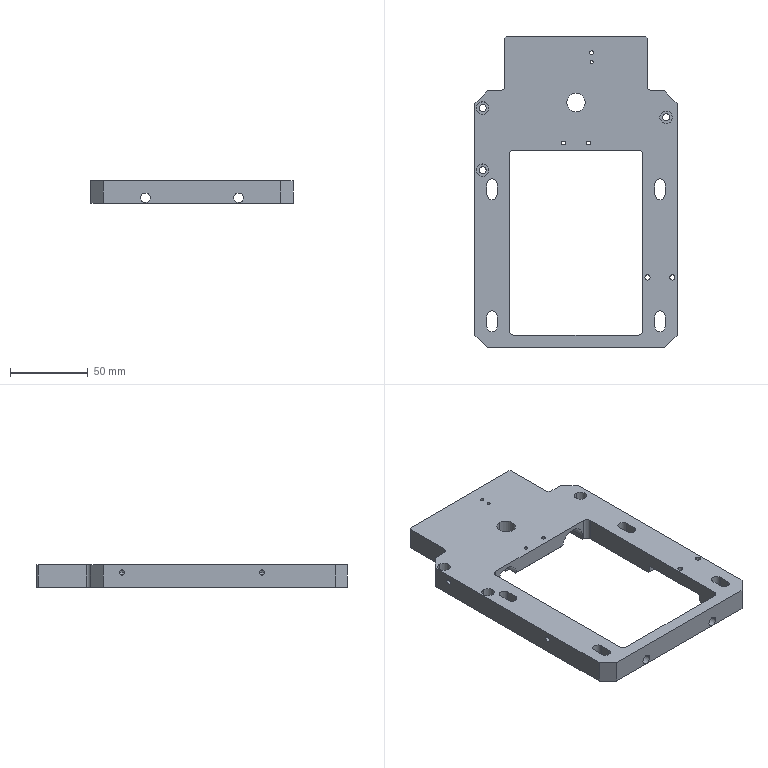NC program | NX | posted with a generic post | part box 130 x 200 x 14.5 mm
Lines 88 to 1425 of 25347:
(ZLEVEL_PROFILE_1_COPY , TOOL : D10)
N144 T04 M6
N146 G54
N148 G17 G0 G90 X12. Y-4.438 B0. C0. S3500 M3
N150 G43 Z30. H4
N152 Z1.5
N154 G94 G1 Y27.952 Z-0.197 F1000.
N156 X12.002 Y28. Z-0.2
N158 X-73.964 F2200.
N160 X-73.976 Y28.003
N162 X-74.442 Y28.002
N164 X-74.46 Y28.004
N166 X-74.993 Y28.
N168 X-77.
N170 Y-28.
N172 X12.002
N174 X12.003 Y-26.135
N176 X12. Y-26.122
N178 Y27.952
N180 X12.002 Y28.
N182 X0.544 Z-0.4
N184 X-73.964
N186 X-73.976 Y28.003
N188 X-74.442 Y28.002
N190 X-74.46 Y28.004
N192 X-74.993 Y28.
N194 X-77.
N196 Y-28.
N198 X12.002
N200 X12.003 Y-26.135
N202 X12. Y-26.122
N204 Y27.952
N206 X12.002 Y28.
N208 X0.544 Z-0.6
N210 X-73.964
N212 X-73.976 Y28.003
N214 X-74.442 Y28.002
N216 X-74.46 Y28.004
N218 X-74.993 Y28.
N220 X-77.
N222 Y-28.
N224 X12.002
N226 X12.003 Y-26.135
N228 X12. Y-26.122
N230 Y27.952
N232 X12.002 Y28.
N234 X0.544 Z-0.8
N236 X-73.964
N238 X-73.976 Y28.003
N240 X-74.442 Y28.002
N242 X-74.46 Y28.004
N244 X-74.993 Y28.
N246 X-77.
N248 Y-28.
N250 X12.002
N252 X12.003 Y-26.135
N254 X12. Y-26.122
N256 Y27.952
N258 X12.002 Y28.
N260 X0.544 Z-1.
N262 X-73.964
N264 X-73.976 Y28.003
N266 X-74.442 Y28.002
N268 X-74.46 Y28.004
N270 X-74.993 Y28.
N272 X-77.
N274 Y-28.
N276 X12.002
N278 X12.003 Y-26.135
N280 X12. Y-26.122
N282 Y27.952
N284 X12.002 Y28.
N286 X0.544 Z-1.2
N288 X-77.
N290 Y-28.
N292 X12.002
N294 X12.003 Y-26.135
N296 X12. Y-26.122
N298 Y27.952
N300 X12.002 Y28.
N302 X0.544 Z-1.4
N304 X-77.
N306 Y-28.
N308 X12.002
N310 X12.003 Y-26.135
N312 X12. Y-26.122
N314 Y27.952
N316 X12.002 Y28.
N318 X0.544 Z-1.6
N320 X-77.
N322 Y-28.
N324 X12.002
N326 X12.003 Y-26.135
N328 X12. Y-26.122
N330 Y27.952
N332 X12.002 Y28.
N334 X0.544 Z-1.8
N336 X-77.
N338 Y-28.
N340 X12.002
N342 X12.003 Y-26.135
N344 X12. Y-26.122
N346 Y27.952
N348 X12.002 Y28.
N350 X0.544 Z-2.
N352 X-77.
N354 Y-28.
N356 X12.002
N358 X12.003 Y-26.135
N360 X12. Y-26.122
N362 Y27.952
N364 X12.002 Y28.
N366 X0.544 Z-2.2
N368 X-77.
N370 Y-28.
N372 X12.002
N374 X12.003 Y-26.135
N376 X12. Y-26.122
N378 Y27.952
N380 X12.002 Y28.
N382 X0.544 Z-2.4
N384 X-77.
N386 Y-28.
N388 X12.002
N390 X12.003 Y-26.135
N392 X12. Y-26.122
N394 Y27.952
N396 X12.002 Y28.
N398 X0.544 Z-2.6
N400 X-77.
N402 Y-28.
N404 X12.002
N406 X12.003 Y-26.135
N408 X12. Y-26.122
N410 Y27.952
N412 X12.002 Y28.
N414 X0.544 Z-2.8
N416 X-77.
N418 Y-28.
N420 X12.002
N422 X12.003 Y-26.135
N424 X12. Y-26.122
N426 Y27.952
N428 X12.002 Y28.
N430 X0.544 Z-3.
N432 X-77.
N434 Y-28.
N436 X12.002
N438 X12.003 Y-26.135
N440 X12. Y-26.122
N442 Y27.952
N444 X12.002 Y28.
N446 X0.544 Z-3.2
N448 X-77.
N450 Y-28.
N452 X12.002
N454 X12.003 Y-26.135
N456 X12. Y-26.122
N458 Y27.952
N460 X12.002 Y28.
N462 X0.544 Z-3.4
N464 X-77.
N466 Y-28.
N468 X12.002
N470 X12.003 Y-26.135
N472 X12. Y-26.122
N474 Y27.952
N476 X12.002 Y28.
N478 X0.544 Z-3.6
N480 X-77.
N482 Y-28.
N484 X12.002
N486 X12.003 Y-26.135
N488 X12. Y-26.122
N490 Y27.952
N492 X12.002 Y28.
N494 X0.544 Z-3.8
N496 X-77.
N498 Y-28.
N500 X12.002
N502 X12.003 Y-26.135
N504 X12. Y-26.122
N506 Y27.952
N508 X12.002 Y28.
N510 X0.544 Z-4.
N512 X-77.
N514 Y-28.
N516 X12.002
N518 X12.003 Y-26.135
N520 X12. Y-26.122
N522 Y27.952
N524 X12.002 Y28.
N526 X0.544 Z-4.2
N528 X-77.
N530 Y-28.
N532 X12.002
N534 X12.003 Y-26.135
N536 X12. Y-26.122
N538 Y27.952
N540 X12.002 Y28.
N542 X0.544 Z-4.4
N544 X-77.
N546 Y-28.
N548 X12.002
N550 X12.003 Y-26.135
N552 X12. Y-26.122
N554 Y27.952
N556 X12.002 Y28.
N558 X0.544 Z-4.6
N560 X-77.
N562 Y-28.
N564 X12.002
N566 X12.003 Y-26.135
N568 X12. Y-26.122
N570 Y27.952
N572 X12.002 Y28.
N574 X0.544 Z-4.8
N576 X-77.
N578 Y-28.
N580 X12.002
N582 X12.003 Y-26.135
N584 X12. Y-26.122
N586 Y27.952
N588 X12.002 Y28.
N590 X0.544 Z-5.
N592 X-77.
N594 Y-28.
N596 X12.002
N598 X12.003 Y-26.135
N600 X12. Y-26.122
N602 Y27.952
N604 X12.002 Y28.
N606 X0.544 Z-5.2
N608 X-77.
N610 Y-28.
N612 X12.002
N614 X12.003 Y-26.135
N616 X12. Y-26.122
N618 Y27.952
N620 X12.002 Y28.
N622 X0.544 Z-5.4
N624 X-77.
N626 Y-28.
N628 X12.002
N630 X12.003 Y-26.135
N632 X12. Y-26.122
N634 Y27.952
N636 X12.002 Y28.
N638 X0.544 Z-5.6
N640 X-77.
N642 Y-28.
N644 X12.002
N646 X12.003 Y-26.135
N648 X12. Y-26.122
N650 Y27.952
N652 X12.002 Y28.
N654 X0.544 Z-5.8
N656 X-77.
N658 Y-28.
N660 X12.002
N662 X12.003 Y-26.135
N664 X12. Y-26.122
N666 Y27.952
N668 X12.002 Y28.
N670 X0.544 Z-6.
N672 X-77.
N674 Y-28.
N676 X12.002
N678 X12.003 Y-26.135
N680 X12. Y-26.122
N682 Y27.952
N684 X12.002 Y28.
N686 X0.544 Z-6.2
N688 X-77.
N690 Y-28.
N692 X12.002
N694 X12.003 Y-26.135
N696 X12. Y-26.122
N698 Y27.952
N700 X12.002 Y28.
N702 X0.544 Z-6.4
N704 X-77.
N706 Y-28.
N708 X12.002
N710 X12.003 Y-26.135
N712 X12. Y-26.122
N714 Y27.952
N716 X12.002 Y28.
N718 X0.544 Z-6.6
N720 X-77.
N722 Y-28.
N724 X12.002
N726 X12.003 Y-26.135
N728 X12. Y-26.122
N730 Y27.952
N732 X12.002 Y28.
N734 X0.544 Z-6.8
N736 X-77.
N738 Y-28.
N740 X12.002
N742 X12.003 Y-26.135
N744 X12. Y-26.122
N746 Y27.952
N748 X12.002 Y28.
N750 X0.544 Z-7.
N752 X-77.
N754 Y-28.
N756 X12.002
N758 X12.003 Y-26.135
N760 X12. Y-26.122
N762 Y27.952
N764 X12.002 Y28.
N766 X0.544 Z-7.2
N768 X-77.
N770 Y-28.
N772 X12.002
N774 X12.003 Y-26.135
N776 X12. Y-26.122
N778 Y27.952
N780 X12.002 Y28.
N782 X0.544 Z-7.4
N784 X-77.
N786 Y-28.
N788 X12.002
N790 X12.003 Y-26.135
N792 X12. Y-26.122
N794 Y27.952
N796 X12.002 Y28.
N798 X0.544 Z-7.6
N800 X-77.
N802 Y-28.
N804 X12.002
N806 X12.003 Y-26.135
N808 X12. Y-26.122
N810 Y27.952
N812 X12.002 Y28.
N814 X0.544 Z-7.8
N816 X-77.
N818 Y-28.
N820 X12.002
N822 X12.003 Y-26.135
N824 X12. Y-26.122
N826 Y27.952
N828 X12.002 Y28.
N830 X0.544 Z-8.
N832 X-77.
N834 Y-28.
N836 X12.002
N838 X12.003 Y-26.135
N840 X12. Y-26.122
N842 Y27.952
N844 X12.002 Y28.
N846 X0.544 Z-8.2
N848 X-77.
N850 Y-28.
N852 X12.002
N854 X12.003 Y-26.135
N856 X12. Y-26.122
N858 Y27.952
N860 X12.002 Y28.
N862 X0.544 Z-8.4
N864 X-77.
N866 Y-28.
N868 X12.002
N870 X12.003 Y-26.135
N872 X12. Y-26.122
N874 Y27.952
N876 X12.002 Y28.
N878 X0.544 Z-8.6
N880 X-77.
N882 Y-28.
N884 X12.002
N886 X12.003 Y-26.135
N888 X12. Y-26.122
N890 Y27.952
N892 X12.002 Y28.
N894 X0.544 Z-8.8
N896 X-77.
N898 Y-28.
N900 X12.002
N902 X12.003 Y-26.135
N904 X12. Y-26.122
N906 Y27.952
N908 X12.002 Y28.
N910 X0.544 Z-9.
N912 X-77.
N914 Y-28.
N916 X12.002
N918 X12.003 Y-26.135
N920 X12. Y-26.122
N922 Y27.952
N924 X12.002 Y28.
N926 X0.544 Z-9.2
N928 X-77.
N930 Y-28.
N932 X12.002
N934 X12.003 Y-26.135
N936 X12. Y-26.122
N938 Y27.952
N940 X12.002 Y28.
N942 X0.544 Z-9.4
N944 X-77.
N946 Y-28.
N948 X12.002
N950 X12.003 Y-26.135
N952 X12. Y-26.122
N954 Y27.952
N956 X12.002 Y28.
N958 X0.544 Z-9.6
N960 X-77.
N962 Y-28.
N964 X12.002
N966 Y-26.135
N968 X12. Y-26.122
N970 Y27.952
N972 X12.002 Y28.
N974 X0.544 Z-9.8
N976 X-77.
N978 Y-28.
N980 X12.002
N982 Y-26.135
N984 X12. Y-26.122
N986 Y27.952
N988 X12.002 Y28.
N990 X0.544 Z-10.
N992 X-77.
N994 Y-28.
N996 X12.002
N998 Y-26.135
N1000 X12. Y-26.122
N1002 Y27.952
N1004 X12.002 Y28.
N1006 X0.544 Z-10.2
N1008 X-77.
N1010 Y-28.
N1012 X12.002
N1014 Y-26.135
N1016 X12. Y-26.122
N1018 Y27.952
N1020 X12.002 Y28.
N1022 X0.544 Z-10.4
N1024 X-77.
N1026 Y-28.
N1028 X12.002
N1030 Y-26.135
N1032 X12. Y-26.122
N1034 Y27.952
N1036 X12.002 Y28.
N1038 X0.544 Z-10.6
N1040 X-77.
N1042 Y-28.
N1044 X12.002
N1046 Y-26.135
N1048 X12. Y-26.122
N1050 Y27.952
N1052 X12.002 Y28.
N1054 X0.544 Z-10.8
N1056 X-77.
N1058 Y-28.
N1060 X12.002
N1062 Y-26.135
N1064 X12. Y-26.122
N1066 Y27.952
N1068 X12.002 Y28.
N1070 X0.544 Z-11.
N1072 X-77.
N1074 Y-28.
N1076 X12.002
N1078 Y-26.135
N1080 X12. Y-26.122
N1082 Y27.952
N1084 X12.002 Y28.
N1086 X0.544 Z-11.2
N1088 X-77.
N1090 Y-28.
N1092 X12.002
N1094 X12. Y-26.313
N1096 Y27.952
N1098 X12.002 Y28.
N1100 X0.544 Z-11.4
N1102 X-77.
N1104 Y-28.
N1106 X12.002
N1108 X12. Y-26.772
N1110 Y27.952
N1112 X12.002 Y28.
N1114 X0.544 Z-11.6
N1116 X-77.
N1118 Y-28.
N1120 X12.002
N1122 Y-27.426
N1124 X12. Y-27.369
N1126 Y27.952
N1128 X12.002 Y28.
N1130 X0.544 Z-11.8
N1132 X-77.
N1134 Y-28.
N1136 X12.002
N1138 X12. Y-27.952
N1140 Y27.952
N1142 X12.002 Y28.
N1144 X0.544 Z-12.
N1146 X-77.
N1148 Y-28.
N1150 X12.002
N1152 X12. Y-27.952
N1154 Y27.952
N1156 X12.002 Y28.
N1158 X0.544 Z-12.2
N1160 X-77.
N1162 Y-28.
N1164 X12.002
N1166 X12. Y-27.952
N1168 Y27.952
N1170 X12.002 Y28.
N1172 X0.544 Z-12.4
N1174 X-77.
N1176 Y-28.
N1178 X12.002
N1180 X12. Y-27.952
N1182 Y27.952
N1184 X12.002 Y28.
N1186 X0.544 Z-12.6
N1188 X-77.
N1190 Y-28.
N1192 X12.002
N1194 X12. Y-27.952
N1196 Y27.952
N1198 X12.002 Y28.
N1200 X0.544 Z-12.8
N1202 X-77.
N1204 Y-28.
N1206 X12.002
N1208 X12. Y-27.952
N1210 Y27.952
N1212 X12.002 Y28.
N1214 X0.544 Z-13.
N1216 X-77.
N1218 Y-28.
N1220 X12.002
N1222 X12. Y-27.952
N1224 Y27.952
N1226 X12.002 Y28.
N1228 X0.544 Z-13.2
N1230 X-77.
N1232 Y-28.
N1234 X12.002
N1236 X12. Y-27.952
N1238 Y27.952
N1240 X12.002 Y28.
N1242 X0.544 Z-13.4
N1244 X-77.
N1246 Y-28.
N1248 X12.002
N1250 X12. Y-27.952
N1252 Y27.952
N1254 X12.002 Y28.
N1256 X0.544 Z-13.6
N1258 X-77.
N1260 Y-28.
N1262 X12.002
N1264 X12. Y-27.952
N1266 Y27.952
N1268 X12.002 Y28.
N1270 X1.26 Z-13.788
N1272 X-77.
N1274 Y-28.
N1276 X12.002
N1278 X12. Y-27.952
N1280 Y27.952
N1282 X12.002 Y28.
N1284 X1.26 Z-13.975
N1286 X-77.
N1288 Y-28.
N1290 X12.002
N1292 X12. Y-27.952
N1294 Y27.952
N1296 X12.002 Y28.
N1298 X1.26 Z-14.163
N1300 X-77.
N1302 Y-28.
N1304 X12.002
N1306 X12. Y-27.952
N1308 Y27.952
N1310 X12.002 Y28.
N1312 X1.26 Z-14.35
N1314 X-77.
N1316 Y-28.
N1318 X12.002
N1320 X12. Y-27.952
N1322 Y27.952
N1324 X12.002 Y28.
N1326 X1.26
N1328 Z-12.85
N1330 G0 Z30.
(ZLEVEL_PROFILE_1 , TOOL : D10)
N1332 X21.9 Y5.462
N1334 Z1.5
N1336 G1 Y37.875 Z-0.199 F1000.
N1338 X21.903 Y37.9 Z-0.2
N1340 X-74.386 F2200.
N1342 X-74.4 Y37.903
N1344 X-74.668 Y37.904
N1346 X-74.99 Y37.9
N1348 X-86.9
N1350 Y-37.9
N1352 X21.903
N1354 X21.9 Y-37.875
N1356 Y37.875
N1358 X21.903 Y37.9
N1360 X10.445 Z-0.4
N1362 X-74.386
N1364 X-74.4 Y37.903
N1366 X-74.668 Y37.904
N1368 X-74.99 Y37.9
N1370 X-86.9
N1372 Y-37.9
N1374 X21.903
N1376 X21.9 Y-37.875
N1378 Y37.875
N1380 X21.903 Y37.9
N1382 X10.445 Z-0.6
N1384 X-74.386
N1386 X-74.4 Y37.903
N1388 X-74.668 Y37.904
N1390 X-74.99 Y37.9
N1392 X-86.9
N1394 Y-37.9
N1396 X21.903
N1398 X21.9 Y-37.875
N1400 Y37.875
N1402 X21.903 Y37.9
N1404 X10.445 Z-0.8
N1406 X-74.386
N1408 X-74.4 Y37.903
N1410 X-74.668 Y37.904
N1412 X-74.99 Y37.9
N1414 X-86.9
N1416 Y-37.9
N1418 X21.903
N1420 X21.9 Y-37.875
N1422 Y37.875
N1424 X21.903 Y37.9
N1426 X10.445 Z-1.
N1428 X-74.386
N1430 X-74.4 Y37.903
N1432 X-74.668 Y37.904
N1434 X-74.99 Y37.9
N1436 X-86.9
N1438 Y-37.9
N1440 X21.903
N1442 X21.9 Y-37.875
N1444 Y37.875
N1446 X21.903 Y37.9
N1448 X10.445 Z-1.2
N1450 X-86.9
N1452 Y-37.9
N1454 X21.903
N1456 X21.9 Y-37.875
N1458 Y37.875
N1460 X21.903 Y37.9
N1462 X10.445 Z-1.4
N1464 X-86.9
N1466 Y-37.9
N1468 X21.903
N1470 X21.9 Y-37.875
N1472 Y37.875
N1474 X21.903 Y37.9
N1476 X10.445 Z-1.6
N1478 X-86.9
N1480 Y-37.9
N1482 X21.903
N1484 X21.9 Y-37.875
N1486 Y37.875
N1488 X21.903 Y37.9
N1490 X10.445 Z-1.8
N1492 X-86.9
N1494 Y-37.9
N1496 X21.903
N1498 X21.9 Y-37.875
N1500 Y37.875
N1502 X21.903 Y37.9
N1504 X10.445 Z-2.
N1506 X-86.9
N1508 Y-37.9
N1510 X21.903
N1512 X21.9 Y-37.875
N1514 Y37.875
N1516 X21.903 Y37.9
N1518 X10.445 Z-2.2
N1520 X-86.9
N1522 Y-37.9
N1524 X21.903
N1526 X21.9 Y-37.875
N1528 Y37.875
N1530 X21.903 Y37.9
N1532 X10.445 Z-2.4
N1534 X-86.9
N1536 Y-37.9
N1538 X21.903
N1540 X21.9 Y-37.875
N1542 Y37.875
N1544 X21.903 Y37.9
N1546 X10.445 Z-2.6
N1548 X-86.9
N1550 Y-37.9
N1552 X21.903
N1554 X21.9 Y-37.875
N1556 Y37.875
N1558 X21.903 Y37.9
N1560 X10.445 Z-2.8
N1562 X-86.9
N1564 Y-37.9
N1566 X21.903
N1568 X21.9 Y-37.875
N1570 Y37.875
N1572 X21.903 Y37.9
N1574 X10.445 Z-3.
N1576 X-86.9
N1578 Y-37.9
N1580 X21.903
N1582 X21.9 Y-37.875
N1584 Y37.875
N1586 X21.903 Y37.9
N1588 X10.445 Z-3.2
N1590 X-86.9
N1592 Y-37.9
N1594 X21.903
N1596 X21.9 Y-37.875
N1598 Y37.875
N1600 X21.903 Y37.9
N1602 X10.445 Z-3.4
N1604 X-86.9
N1606 Y-37.9
N1608 X21.903
N1610 X21.9 Y-37.875
N1612 Y37.875
N1614 X21.903 Y37.9
N1616 X10.445 Z-3.6
N1618 X-86.9
N1620 Y-37.9
N1622 X21.903
N1624 X21.9 Y-37.875
N1626 Y37.875
N1628 X21.903 Y37.9
N1630 X10.445 Z-3.8
N1632 X-86.9
N1634 Y-37.9
N1636 X21.903
N1638 X21.9 Y-37.875
N1640 Y37.875
N1642 X21.903 Y37.9
N1644 X10.445 Z-4.
N1646 X-86.9
N1648 Y-37.9
N1650 X21.903
N1652 X21.9 Y-37.875
N1654 Y37.875
N1656 X21.903 Y37.9
N1658 X10.445 Z-4.2
N1660 X-86.9
N1662 Y-37.9
N1664 X21.903
N1666 X21.9 Y-37.875
N1668 Y37.875
N1670 X21.903 Y37.9
N1672 X10.445 Z-4.4
N1674 X-86.9
N1676 Y-37.9
N1678 X21.903
N1680 X21.9 Y-37.875
N1682 Y37.875
N1684 X21.903 Y37.9
N1686 X10.445 Z-4.6
N1688 X-86.9
N1690 Y-37.9
N1692 X21.903
N1694 X21.9 Y-37.875
N1696 Y37.875
N1698 X21.903 Y37.9
N1700 X10.445 Z-4.8
N1702 X-86.9
N1704 Y-37.9
N1706 X21.903
N1708 X21.9 Y-37.875
N1710 Y37.875
N1712 X21.903 Y37.9
N1714 X10.445 Z-5.
N1716 X-86.9
N1718 Y-37.9
N1720 X21.903
N1722 X21.9 Y-37.875
N1724 Y37.875
N1726 X21.903 Y37.9
N1728 X10.445 Z-5.2
N1730 X-86.9
N1732 Y-37.9
N1734 X21.903
N1736 X21.9 Y-37.875
N1738 Y37.875
N1740 X21.903 Y37.9
N1742 X10.445 Z-5.4
N1744 X-86.9
N1746 Y-37.9
N1748 X21.903
N1750 X21.9 Y-37.875
N1752 Y37.875
N1754 X21.903 Y37.9
N1756 X10.445 Z-5.6
N1758 X-86.9
N1760 Y-37.9
N1762 X21.903
N1764 X21.9 Y-37.875
N1766 Y37.875
N1768 X21.903 Y37.9
N1770 X10.445 Z-5.8
N1772 X-86.9
N1774 Y-37.9
N1776 X21.903
N1778 X21.9 Y-37.875
N1780 Y37.875
N1782 X21.903 Y37.9
N1784 X10.445 Z-6.
N1786 X-86.9
N1788 Y-37.9
N1790 X21.903
N1792 X21.9 Y-37.875
N1794 Y37.875
N1796 X21.903 Y37.9
N1798 X10.445 Z-6.2
N1800 X-86.9
N1802 Y-37.9
N1804 X21.903
N1806 X21.9 Y-37.875
N1808 Y37.875
N1810 X21.903 Y37.9
N1812 X10.445 Z-6.4
N1814 X-86.9
N1816 Y-37.9
N1818 X21.903
N1820 X21.9 Y-37.875
N1822 Y37.875
N1824 X21.903 Y37.9
N1826 X10.445 Z-6.6
N1828 X-86.9
N1830 Y-37.9
N1832 X21.903
N1834 X21.9 Y-37.875
N1836 Y37.875
N1838 X21.903 Y37.9
N1840 X10.445 Z-6.8
N1842 X-86.9
N1844 Y-37.9
N1846 X21.903
N1848 X21.9 Y-37.875
N1850 Y37.875
N1852 X21.903 Y37.9
N1854 X10.445 Z-7.
N1856 X-86.9
N1858 Y-37.9
N1860 X21.903
N1862 X21.9 Y-37.875
N1864 Y37.875
N1866 X21.903 Y37.9
N1868 X10.445 Z-7.2
N1870 X-86.9
N1872 Y-37.9
N1874 X21.903
N1876 X21.9 Y-37.875
N1878 Y37.875
N1880 X21.903 Y37.9
N1882 X10.445 Z-7.4
N1884 X-86.9
N1886 Y-37.9
N1888 X21.903
N1890 X21.9 Y-37.873
N1892 Y37.873
N1894 X21.903 Y37.9
N1896 X10.445 Z-7.6
N1898 X-86.9
N1900 Y-37.9
N1902 X21.903
N1904 X21.9 Y-37.873
N1906 Y37.873
N1908 X21.903 Y37.9
N1910 X10.445 Z-7.8
N1912 X-86.9
N1914 Y-37.9
N1916 X21.903
N1918 X21.9 Y-37.873
N1920 Y37.873
N1922 X21.903 Y37.9
N1924 X10.445 Z-8.
N1926 X-86.9
N1928 Y-37.9
N1930 X21.903
N1932 X21.9 Y-37.873
N1934 Y37.873
N1936 X21.903 Y37.9
N1938 X10.445 Z-8.2
N1940 X-86.9
N1942 Y-37.9
N1944 X21.903
N1946 X21.9 Y-37.873
N1948 Y37.873
N1950 X21.903 Y37.9
N1952 X10.445 Z-8.4
N1954 X-86.9
N1956 Y-37.9
N1958 X21.903
N1960 X21.9 Y-37.873
N1962 Y37.873
N1964 X21.903 Y37.9
N1966 X10.445 Z-8.6
N1968 X-86.9
N1970 Y-37.9
N1972 X21.903
N1974 X21.9 Y-37.873
N1976 Y37.873
N1978 X21.903 Y37.9
N1980 X10.445 Z-8.8
N1982 X-86.9
N1984 Y-37.9
N1986 X21.903
N1988 X21.9 Y-37.873
N1990 Y37.873
N1992 X21.903 Y37.9
N1994 X10.445 Z-9.
N1996 X-86.9
N1998 Y-37.9
N2000 X21.903
N2002 X21.9 Y-37.873
N2004 Y37.873
N2006 X21.903 Y37.9
N2008 X10.445 Z-9.2
N2010 X-86.9
N2012 Y-37.9
N2014 X21.903
N2016 X21.9 Y-37.873
N2018 Y37.873
N2020 X21.903 Y37.9
N2022 X10.445 Z-9.4
N2024 X-86.9
N2026 Y-37.9
N2028 X21.903
N2030 X21.9 Y-37.873
N2032 Y37.873
N2034 X21.903 Y37.9
N2036 X10.445 Z-9.6
N2038 X-86.9
N2040 Y-37.9
N2042 X21.903
N2044 X21.9 Y-37.873
N2046 Y37.873
N2048 X21.903 Y37.9
N2050 X10.445 Z-9.8
N2052 X-86.9
N2054 Y-37.9
N2056 X21.903
N2058 X21.9 Y-37.873
N2060 Y37.873
N2062 X21.903 Y37.9
N2064 X10.445 Z-10.
N2066 X-86.9
N2068 Y-37.9
N2070 X21.903
N2072 X21.9 Y-37.873
N2074 Y37.873
N2076 X21.903 Y37.9
N2078 X10.445 Z-10.2
N2080 X-86.9
N2082 Y-37.9
N2084 X21.903
N2086 X21.9 Y-37.873
N2088 Y37.873
N2090 X21.903 Y37.9
N2092 X10.445 Z-10.4
N2094 X-86.9
N2096 Y-37.9
N2098 X21.903
N2100 X21.9 Y-37.873
N2102 Y37.873
N2104 X21.903 Y37.9
N2106 X10.445 Z-10.6
N2108 X-86.9
N2110 Y-37.9
N2112 X21.903
N2114 X21.9 Y-37.873
N2116 Y37.873
N2118 X21.903 Y37.9
N2120 X10.445 Z-10.8
N2122 X-86.9
N2124 Y-37.9
N2126 X21.903
N2128 X21.9 Y-37.873
N2130 Y37.873
N2132 X21.903 Y37.9
N2134 X10.445 Z-11.
N2136 X-86.9
N2138 Y-37.9
N2140 X21.903
N2142 X21.9 Y-37.873
N2144 Y37.873
N2146 X21.903 Y37.9
N2148 X10.445 Z-11.2
N2150 X-86.9
N2152 Y-37.9
N2154 X21.903
N2156 X21.9 Y-37.873
N2158 Y37.873
N2160 X21.903 Y37.9
N2162 X10.445 Z-11.4
N2164 X-86.9
N2166 Y-37.9
N2168 X21.903
N2170 X21.9 Y-37.873
N2172 Y37.873
N2174 X21.903 Y37.9
N2176 X10.445 Z-11.6
N2178 X-86.9
N2180 Y-37.9
N2182 X21.903
N2184 X21.9 Y-37.873
N2186 Y37.873
N2188 X21.903 Y37.9
N2190 X10.445 Z-11.8
N2192 X-86.9
N2194 Y-37.9
N2196 X21.903
N2198 X21.9 Y-37.873
N2200 Y37.873
N2202 X21.903 Y37.9
N2204 X10.445 Z-12.
N2206 X-86.9
N2208 Y-37.9
N2210 X21.903
N2212 X21.9 Y-37.873
N2214 Y37.873
N2216 X21.903 Y37.9
N2218 X10.445 Z-12.2
N2220 X-86.9
N2222 Y-37.9
N2224 X21.903
N2226 X21.9 Y-37.873
N2228 Y37.873
N2230 X21.903 Y37.9
N2232 X10.445 Z-12.4
N2234 X-86.9
N2236 Y-37.9
N2238 X21.903
N2240 X21.9 Y-37.873
N2242 Y37.873
N2244 X21.903 Y37.9
N2246 X10.445 Z-12.6
N2248 X-86.9
N2250 Y-37.9
N2252 X21.903
N2254 X21.9 Y-37.873
N2256 Y37.873
N2258 X21.903 Y37.9
N2260 X10.445 Z-12.8
N2262 X-86.9
N2264 Y-37.9
N2266 X21.903
N2268 X21.9 Y-37.873
N2270 Y37.873
N2272 X21.903 Y37.9
N2274 X10.445 Z-13.
N2276 X-86.9
N2278 Y-37.9
N2280 X21.903
N2282 X21.9 Y-37.873
N2284 Y37.873
N2286 X21.903 Y37.9
N2288 X10.445 Z-13.2
N2290 X-86.9
N2292 Y-37.9
N2294 X21.903
N2296 X21.9 Y-37.873
N2298 Y37.873
N2300 X21.903 Y37.9
N2302 X10.445 Z-13.4
N2304 X-86.9
N2306 Y-37.9
N2308 X21.903
N2310 X21.9 Y-37.873
N2312 Y37.873
N2314 X21.903 Y37.9
N2316 X10.445 Z-13.6
N2318 X-86.9
N2320 Y-37.9
N2322 X21.903
N2324 X21.9 Y-37.873
N2326 Y37.873
N2328 X21.903 Y37.9
N2330 X11.161 Z-13.788
N2332 X-86.9
N2334 Y-37.9
N2336 X21.903
N2338 X21.9 Y-37.873
N2340 Y37.873
N2342 X21.903 Y37.9
N2344 X11.161 Z-13.975
N2346 X-86.9
N2348 Y-37.9
N2350 X21.903
N2352 X21.9 Y-37.873
N2354 Y37.873
N2356 X21.903 Y37.9
N2358 X11.161 Z-14.163
N2360 X-86.9
N2362 Y-37.9
N2364 X21.903
N2366 X21.9 Y-37.873
N2368 Y37.873
N2370 X21.903 Y37.9
N2372 X11.161 Z-14.35
N2374 X-86.9
N2376 Y-37.9
N2378 X21.903
N2380 X21.9 Y-37.873
N2382 Y37.873
N2384 X21.903 Y37.9
N2386 X11.161
N2388 Z-12.85
N2390 G0 Z30.
(ZLEVEL_PROFILE , TOOL : D10)
N2392 X-91.876 Y-74.907
N2394 Z-0.22
N2396 G1 X-91.482 Y-73.434 F1000.
N2398 G3 X-91.741 Y-72.469 R1.
N2400 G1 X-95.585 Y-68.627 F2200.
N2402 X-102.637 Y-61.575
N2404 X-103.21 Y-61.
N2406 X-103.199 Y-60.972
N2408 G2 X-104.117 Y-60.01 R5.1
N2410 G1 X-104.193 Y-60.019
N2412 X-107.469 Y-56.741
N2414 G3 X-108.434 Y-56.482 R1.
N2416 G1 X-109.907 Y-56.876
N2418 G0 Z-0.439
N2420 G1 X-108.434 Y-56.482 F1000.
N2422 G2 X-107.469 Y-56.741 R1.
N2424 G1 X-104.193 Y-60.019 F2200.
N2426 X-104.117 Y-60.01
N2428 G3 X-103.199 Y-60.972 R5.1
N2430 G1 X-103.21 Y-61.
N2432 X-102.637 Y-61.575
N2434 X-95.585 Y-68.627
N2436 X-91.741 Y-72.469
N2438 G2 X-91.482 Y-73.434 R1.
N2440 G1 X-91.876 Y-74.907
N2442 G0 Z-0.659
N2444 G1 X-91.482 Y-73.434 F1000.
N2446 G3 X-91.741 Y-72.469 R1.
N2448 G1 X-95.585 Y-68.627 F2200.
N2450 X-102.637 Y-61.575
N2452 X-103.21 Y-61.
N2454 X-103.199 Y-60.972
N2456 G2 X-104.117 Y-60.01 R5.1
N2458 G1 X-104.193 Y-60.019
N2460 X-107.469 Y-56.741
N2462 G3 X-108.434 Y-56.482 R1.
N2464 G1 X-109.907 Y-56.876
N2466 G0 Z-0.879
N2468 G1 X-108.434 Y-56.482 F1000.
N2470 G2 X-107.469 Y-56.741 R1.
N2472 G1 X-104.193 Y-60.019 F2200.
N2474 X-104.117 Y-60.01
N2476 G3 X-103.199 Y-60.972 R5.1
N2478 G1 X-103.21 Y-61.
N2480 X-102.637 Y-61.575
N2482 X-95.585 Y-68.627
N2484 X-91.741 Y-72.469
N2486 G2 X-91.482 Y-73.434 R1.
N2488 G1 X-91.876 Y-74.907
N2490 G0 Z-1.098
N2492 G1 X-91.482 Y-73.434 F1000.
N2494 G3 X-91.741 Y-72.469 R1.
N2496 G1 X-95.585 Y-68.627 F2200.
N2498 X-102.637 Y-61.575
N2500 X-103.21 Y-61.
N2502 X-103.199 Y-60.972
N2504 G2 X-104.117 Y-60.01 R5.1
N2506 G1 X-104.193 Y-60.019
N2508 X-107.469 Y-56.741
N2510 G3 X-108.434 Y-56.482 R1.
N2512 G1 X-109.907 Y-56.876
N2514 G0 Z-1.318
N2516 G1 X-108.434 Y-56.482 F1000.
N2518 G2 X-107.469 Y-56.741 R1.
N2520 G1 X-104.193 Y-60.019 F2200.
N2522 X-104.117 Y-60.01
N2524 G3 X-103.199 Y-60.972 R5.1
N2526 G1 X-103.21 Y-61.
N2528 X-102.637 Y-61.575
N2530 X-95.585 Y-68.627
N2532 X-91.741 Y-72.469
N2534 G2 X-91.482 Y-73.434 R1.
N2536 G1 X-91.876 Y-74.907
N2538 G0 Z-1.538
N2540 G1 X-91.482 Y-73.434 F1000.
N2542 G3 X-91.741 Y-72.469 R1.
N2544 G1 X-95.585 Y-68.627 F2200.
N2546 X-102.637 Y-61.575
N2548 X-103.21 Y-61.
N2550 X-103.199 Y-60.972
N2552 G2 X-104.117 Y-60.01 R5.1
N2554 G1 X-104.193 Y-60.019
N2556 X-107.469 Y-56.741
N2558 G3 X-108.434 Y-56.482 R1.
N2560 G1 X-109.907 Y-56.876
N2562 G0 Z-1.758
N2564 G1 X-108.434 Y-56.482 F1000.
N2566 G2 X-107.469 Y-56.741 R1.
N2568 G1 X-104.193 Y-60.019 F2200.
N2570 X-104.117 Y-60.01
N2572 G3 X-103.199 Y-60.972 R5.1
N2574 G1 X-103.21 Y-61.
N2576 X-102.637 Y-61.575
N2578 X-95.585 Y-68.627
N2580 X-91.741 Y-72.469
N2582 G2 X-91.482 Y-73.434 R1.
N2584 G1 X-91.876 Y-74.907
N2586 G0 Z-1.977
N2588 G1 X-91.482 Y-73.434 F1000.
N2590 G3 X-91.741 Y-72.469 R1.
N2592 G1 X-95.585 Y-68.627 F2200.
N2594 X-102.637 Y-61.575
N2596 X-103.21 Y-61.
N2598 X-103.199 Y-60.972
N2600 G2 X-104.117 Y-60.01 R5.1
N2602 G1 X-104.193 Y-60.019
N2604 X-107.469 Y-56.741
N2606 G3 X-108.434 Y-56.482 R1.
N2608 G1 X-109.907 Y-56.876
N2610 G0 Z-2.197
N2612 G1 X-108.435 Y-56.482 F1000.
N2614 G2 X-107.469 Y-56.741 R1.
N2616 G1 X-104.193 Y-60.019 F2200.
N2618 X-104.117 Y-60.01
N2620 G3 X-103.199 Y-60.972 R5.1
N2622 G1 X-103.21 Y-61.
N2624 X-102.637 Y-61.575
N2626 X-95.585 Y-68.627
N2628 X-91.741 Y-72.469
N2630 G2 X-91.482 Y-73.434 R1.
N2632 G1 X-91.876 Y-74.907
N2634 G0 Z-2.417
N2636 G1 X-91.482 Y-73.435 F1000.
N2638 G3 X-91.741 Y-72.469 R1.
N2640 G1 X-95.585 Y-68.627 F2200.
N2642 X-102.637 Y-61.575
N2644 X-103.21 Y-61.
N2646 X-103.199 Y-60.972
N2648 G2 X-104.117 Y-60.01 R5.1
N2650 G1 X-104.193 Y-60.019
N2652 X-107.469 Y-56.741
N2654 G3 X-108.435 Y-56.482 R1.
N2656 G1 X-109.907 Y-56.876
N2658 G0 Z-2.636
N2660 G1 X-108.435 Y-56.482 F1000.
N2662 G2 X-107.469 Y-56.741 R1.
N2664 G1 X-104.193 Y-60.019 F2200.
N2666 X-104.117 Y-60.01
N2668 G3 X-103.199 Y-60.972 R5.1
N2670 G1 X-103.21 Y-61.
N2672 X-102.637 Y-61.575
N2674 X-95.585 Y-68.627
N2676 X-91.741 Y-72.469
N2678 G2 X-91.482 Y-73.435 R1.
N2680 G1 X-91.876 Y-74.907
N2682 G0 Z-2.856
N2684 G1 X-91.482 Y-73.435 F1000.
N2686 G3 X-91.741 Y-72.469 R1.
N2688 G1 X-95.585 Y-68.627 F2200.
N2690 X-102.637 Y-61.575
N2692 X-103.21 Y-61.
N2694 X-103.199 Y-60.972
N2696 G2 X-104.117 Y-60.01 R5.1
N2698 G1 X-104.193 Y-60.019
N2700 X-107.469 Y-56.741
N2702 G3 X-108.435 Y-56.482 R1.
N2704 G1 X-109.907 Y-56.876
N2706 G0 Z-3.076
N2708 G1 X-108.435 Y-56.482 F1000.
N2710 G2 X-107.469 Y-56.741 R1.
N2712 G1 X-104.193 Y-60.019 F2200.
N2714 X-104.117 Y-60.01
N2716 G3 X-103.199 Y-60.972 R5.1
N2718 G1 X-103.21 Y-61.
N2720 X-102.637 Y-61.575
N2722 X-95.585 Y-68.627
N2724 X-91.741 Y-72.469
N2726 G2 X-91.482 Y-73.435 R1.
N2728 G1 X-91.876 Y-74.907
N2730 G0 Z-3.295
N2732 G1 X-91.482 Y-73.435 F1000.
N2734 G3 X-91.741 Y-72.469 R1.
N2736 G1 X-95.585 Y-68.627 F2200.
N2738 X-102.637 Y-61.575
N2740 X-103.21 Y-61.
N2742 X-103.199 Y-60.972
N2744 G2 X-104.117 Y-60.01 R5.1
N2746 G1 X-104.193 Y-60.019
N2748 X-107.469 Y-56.741
N2750 G3 X-108.435 Y-56.482 R1.
N2752 G1 X-109.907 Y-56.876
N2754 G0 Z-3.515
N2756 G1 X-108.435 Y-56.482 F1000.
N2758 G2 X-107.469 Y-56.741 R1.
N2760 G1 X-104.193 Y-60.019 F2200.
N2762 X-104.117 Y-60.01
N2764 G3 X-103.199 Y-60.972 R5.1
N2766 G1 X-103.21 Y-61.
N2768 X-102.637 Y-61.575
N2770 X-95.585 Y-68.627
N2772 X-91.741 Y-72.469
N2774 G2 X-91.482 Y-73.435 R1.
N2776 G1 X-91.876 Y-74.907
N2778 G0 Z-3.735
N2780 G1 X-91.482 Y-73.435 F1000.
N2782 G3 X-91.741 Y-72.469 R1.
N2784 G1 X-95.585 Y-68.627 F2200.
N2786 X-102.637 Y-61.575
N2788 X-103.21 Y-61.
N2790 X-103.199 Y-60.972
N2792 G2 X-104.117 Y-60.01 R5.1
N2794 G1 X-104.193 Y-60.019
N2796 X-107.469 Y-56.741
N2798 G3 X-108.435 Y-56.482 R1.
N2800 G1 X-109.907 Y-56.876